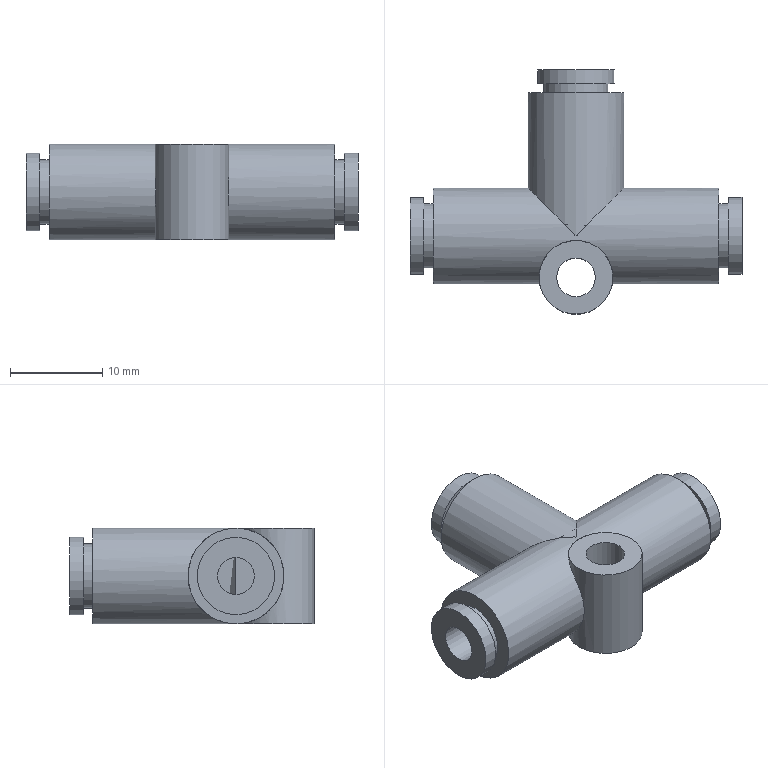Part | NX | 1 solid | 28 faces | box 36 x 26.5 x 10.4 mm | volume 3485 mm3 | plane 14 | cylinder 13 | cone 1 | commonest cylinder face diameters 4 x3 7 x3 8.4 x3 10.4 x2 4.2 x1 8 x1
STEP:
#1=CARTESIAN_POINT('',(0.,0.,5.2));
#2=VERTEX_POINT('',#1);
#3=CARTESIAN_POINT('',(0.,0.,-5.2));
#4=VERTEX_POINT('',#3);
#5=CARTESIAN_POINT('',(0.,0.,0.));
#6=DIRECTION('',(-0.7071,-0.7071,0.));
#7=DIRECTION('',(0.7071,-0.7071,0.));
#8=AXIS2_PLACEMENT_3D('',#5,#6,#7);
#9=ELLIPSE('',#8,7.354,5.2);
#10=EDGE_CURVE('',#2,#4,#9,.T.);
#11=ORIENTED_EDGE('',*,*,#10,.T.);
#12=CARTESIAN_POINT('',(0.,0.,0.));
#13=DIRECTION('',(0.7071,-0.7071,0.));
#14=DIRECTION('',(-0.7071,-0.7071,0.));
#15=AXIS2_PLACEMENT_3D('',#12,#13,#14);
#16=ELLIPSE('',#15,7.354,5.2);
#17=EDGE_CURVE('',#4,#2,#16,.T.);
#18=ORIENTED_EDGE('',*,*,#17,.T.);
#19=EDGE_LOOP('',(#11,#18));
#20=FACE_BOUND('',#19,.T.);
#21=CARTESIAN_POINT('',(-15.5,0.,-5.2));
#22=VERTEX_POINT('',#21);
#23=CARTESIAN_POINT('',(-15.5,0.,0.));
#24=DIRECTION('',(1.,0.,0.));
#25=DIRECTION('',(0.,0.,-1.));
#26=AXIS2_PLACEMENT_3D('',#23,#24,#25);
#27=CIRCLE('',#26,5.2);
#28=EDGE_CURVE('',#22,#22,#27,.T.);
#29=ORIENTED_EDGE('',*,*,#28,.T.);
#30=EDGE_LOOP('',(#29));
#31=FACE_BOUND('',#30,.T.);
#32=CARTESIAN_POINT('',(-4.,-4.5,-2.606));
#33=VERTEX_POINT('',#32);
#34=CARTESIAN_POINT('',(-3.876,-2.858,-4.57));
#35=CARTESIAN_POINT('',(-4.058,-4.689,-2.698));
#36=CARTESIAN_POINT('',(-3.891,-5.385,-0.2717));
#37=CARTESIAN_POINT('',(-4.013,-4.931,2.212));
#38=CARTESIAN_POINT('',(-4.012,-3.327,4.258));
#39=CARTESIAN_POINT('',(-2.719,-1.208,5.153));
#40=CARTESIAN_POINT('',(-0.2808,-0.2446,5.177));
#41=CARTESIAN_POINT('',(2.249,-0.8668,5.188));
#42=CARTESIAN_POINT('',(3.874,-2.854,4.572));
#43=CARTESIAN_POINT('',(4.059,-4.685,2.705));
#44=CARTESIAN_POINT('',(3.891,-5.385,0.2764));
#45=CARTESIAN_POINT('',(4.013,-4.933,-2.209));
#46=CARTESIAN_POINT('',(4.013,-3.329,-4.257));
#47=CARTESIAN_POINT('',(2.72,-1.207,-5.153));
#48=CARTESIAN_POINT('',(0.2792,-0.2442,-5.177));
#49=CARTESIAN_POINT('',(-2.252,-0.8683,-5.188));
#50=CARTESIAN_POINT('',(-3.876,-2.858,-4.57));
#51=CARTESIAN_POINT('',(-4.058,-4.689,-2.698));
#52=CARTESIAN_POINT('',(-3.891,-5.385,-0.2717));
#53=B_SPLINE_CURVE_WITH_KNOTS('',3,(#34,#35,#36,#37,#38,#39,#40,#41,#42,#43,#44,#45,#46,#47,#48,#49,#50,#51,#52),.UNSPECIFIED.,.T.,.F.,(1,1,1,1,1,1,1,1,1,1,1,1,1,1,1,1,1,1,1,1,1,1,1),(-0.01004,-0.007597,-0.00515,-0.002704,-0.0002574,0.002189,0.004636,0.007082,0.009529,0.01198,0.01442,0.01687,0.01931,0.02176,0.02421,0.02665,0.0291,0.03155,0.03399,0.03644,0.03889,0.04133,0.04378),.UNSPECIFIED.);
#54=EDGE_CURVE('',#33,#33,#53,.T.);
#55=ORIENTED_EDGE('',*,*,#54,.T.);
#56=EDGE_LOOP('',(#55));
#57=FACE_BOUND('',#56,.T.);
#58=CARTESIAN_POINT('',(15.5,0.,-5.2));
#59=VERTEX_POINT('',#58);
#60=CARTESIAN_POINT('',(15.5,0.,0.));
#61=DIRECTION('',(1.,0.,0.));
#62=DIRECTION('',(0.,0.,-1.));
#63=AXIS2_PLACEMENT_3D('',#60,#61,#62);
#64=CIRCLE('',#63,5.2);
#65=EDGE_CURVE('',#59,#59,#64,.F.);
#66=ORIENTED_EDGE('',*,*,#65,.T.);
#67=EDGE_LOOP('',(#66));
#68=FACE_BOUND('',#67,.T.);
#69=CARTESIAN_POINT('',(0.,0.,0.));
#70=DIRECTION('',(1.,0.,0.));
#71=DIRECTION('',(0.,0.,-1.));
#72=AXIS2_PLACEMENT_3D('',#69,#70,#71);
#73=CYLINDRICAL_SURFACE('',#72,5.2);
#74=ADVANCED_FACE('',(#20,#31,#57,#68),#73,.T.);
#75=CARTESIAN_POINT('',(15.5,0.,-3.5));
#76=VERTEX_POINT('',#75);
#77=CARTESIAN_POINT('',(15.5,0.,0.));
#78=DIRECTION('',(1.,0.,0.));
#79=DIRECTION('',(0.,0.,-1.));
#80=AXIS2_PLACEMENT_3D('',#77,#78,#79);
#81=CIRCLE('',#80,3.5);
#82=EDGE_CURVE('',#76,#76,#81,.F.);
#83=ORIENTED_EDGE('',*,*,#82,.T.);
#84=EDGE_LOOP('',(#83));
#85=FACE_BOUND('',#84,.T.);
#86=ORIENTED_EDGE('',*,*,#65,.F.);
#87=EDGE_LOOP('',(#86));
#88=FACE_BOUND('',#87,.T.);
#89=CARTESIAN_POINT('',(15.5,4.35,0.));
#90=DIRECTION('',(1.,0.,0.));
#91=DIRECTION('',(0.,0.,-1.));
#92=AXIS2_PLACEMENT_3D('',#89,#90,#91);
#93=PLANE('',#92);
#94=ADVANCED_FACE('',(#85,#88),#93,.T.);
#95=CARTESIAN_POINT('',(4.,-4.5,5.2));
#96=VERTEX_POINT('',#95);
#97=CARTESIAN_POINT('',(0.,-4.5,5.2));
#98=DIRECTION('',(0.,0.,1.));
#99=DIRECTION('',(1.,0.,0.));
#100=AXIS2_PLACEMENT_3D('',#97,#98,#99);
#101=CIRCLE('',#100,4.);
#102=EDGE_CURVE('',#96,#96,#101,.F.);
#103=ORIENTED_EDGE('',*,*,#102,.T.);
#104=EDGE_LOOP('',(#103));
#105=FACE_BOUND('',#104,.T.);
#106=CARTESIAN_POINT('',(4.,-4.5,-5.2));
#107=VERTEX_POINT('',#106);
#108=CARTESIAN_POINT('',(0.,-4.5,-5.2));
#109=DIRECTION('',(0.,0.,1.));
#110=DIRECTION('',(1.,0.,0.));
#111=AXIS2_PLACEMENT_3D('',#108,#109,#110);
#112=CIRCLE('',#111,4.);
#113=EDGE_CURVE('',#107,#107,#112,.T.);
#114=ORIENTED_EDGE('',*,*,#113,.T.);
#115=EDGE_LOOP('',(#114));
#116=FACE_BOUND('',#115,.T.);
#117=ORIENTED_EDGE('',*,*,#54,.F.);
#118=EDGE_LOOP('',(#117));
#119=FACE_BOUND('',#118,.T.);
#120=CARTESIAN_POINT('',(0.,-4.5,5.2));
#121=DIRECTION('',(0.,0.,1.));
#122=DIRECTION('',(1.,0.,0.));
#123=AXIS2_PLACEMENT_3D('',#120,#121,#122);
#124=CYLINDRICAL_SURFACE('',#123,4.);
#125=ADVANCED_FACE('',(#105,#116,#119),#124,.T.);
#126=ORIENTED_EDGE('',*,*,#28,.F.);
#127=EDGE_LOOP('',(#126));
#128=FACE_BOUND('',#127,.T.);
#129=CARTESIAN_POINT('',(-15.5,0.,-3.5));
#130=VERTEX_POINT('',#129);
#131=CARTESIAN_POINT('',(-15.5,0.,0.));
#132=DIRECTION('',(1.,0.,0.));
#133=DIRECTION('',(0.,0.,-1.));
#134=AXIS2_PLACEMENT_3D('',#131,#132,#133);
#135=CIRCLE('',#134,3.5);
#136=EDGE_CURVE('',#130,#130,#135,.T.);
#137=ORIENTED_EDGE('',*,*,#136,.T.);
#138=EDGE_LOOP('',(#137));
#139=FACE_BOUND('',#138,.T.);
#140=CARTESIAN_POINT('',(-15.5,4.35,0.));
#141=DIRECTION('',(-1.,0.,0.));
#142=DIRECTION('',(0.,0.,1.));
#143=AXIS2_PLACEMENT_3D('',#140,#141,#142);
#144=PLANE('',#143);
#145=ADVANCED_FACE('',(#128,#139),#144,.T.);
#146=CARTESIAN_POINT('',(0.,15.5,-5.2));
#147=VERTEX_POINT('',#146);
#148=CARTESIAN_POINT('',(0.,15.5,0.));
#149=DIRECTION('',(0.,-1.,0.));
#150=DIRECTION('',(0.,0.,-1.));
#151=AXIS2_PLACEMENT_3D('',#148,#149,#150);
#152=CIRCLE('',#151,5.2);
#153=EDGE_CURVE('',#147,#147,#152,.T.);
#154=ORIENTED_EDGE('',*,*,#153,.T.);
#155=EDGE_LOOP('',(#154));
#156=FACE_BOUND('',#155,.T.);
#157=ORIENTED_EDGE('',*,*,#10,.F.);
#158=ORIENTED_EDGE('',*,*,#17,.F.);
#159=EDGE_LOOP('',(#157,#158));
#160=FACE_BOUND('',#159,.T.);
#161=CARTESIAN_POINT('',(0.,7.75,0.));
#162=DIRECTION('',(0.,-1.,0.));
#163=DIRECTION('',(0.,0.,-1.));
#164=AXIS2_PLACEMENT_3D('',#161,#162,#163);
#165=CYLINDRICAL_SURFACE('',#164,5.2);
#166=ADVANCED_FACE('',(#156,#160),#165,.T.);
#167=ORIENTED_EDGE('',*,*,#82,.F.);
#168=EDGE_LOOP('',(#167));
#169=FACE_BOUND('',#168,.T.);
#170=CARTESIAN_POINT('',(16.5,0.,-3.5));
#171=VERTEX_POINT('',#170);
#172=CARTESIAN_POINT('',(16.5,0.,0.));
#173=DIRECTION('',(1.,0.,0.));
#174=DIRECTION('',(0.,0.,-1.));
#175=AXIS2_PLACEMENT_3D('',#172,#173,#174);
#176=CIRCLE('',#175,3.5);
#177=EDGE_CURVE('',#171,#171,#176,.F.);
#178=ORIENTED_EDGE('',*,*,#177,.T.);
#179=EDGE_LOOP('',(#178));
#180=FACE_BOUND('',#179,.T.);
#181=CARTESIAN_POINT('',(16.,0.,0.));
#182=DIRECTION('',(1.,0.,0.));
#183=DIRECTION('',(0.,0.,-1.));
#184=AXIS2_PLACEMENT_3D('',#181,#182,#183);
#185=CYLINDRICAL_SURFACE('',#184,3.5);
#186=ADVANCED_FACE('',(#169,#180),#185,.T.);
#187=ORIENTED_EDGE('',*,*,#113,.F.);
#188=EDGE_LOOP('',(#187));
#189=FACE_BOUND('',#188,.T.);
#190=CARTESIAN_POINT('',(2.1,-4.5,-5.2));
#191=VERTEX_POINT('',#190);
#192=CARTESIAN_POINT('',(0.,-4.5,-5.2));
#193=DIRECTION('',(0.,0.,1.));
#194=DIRECTION('',(1.,0.,0.));
#195=AXIS2_PLACEMENT_3D('',#192,#193,#194);
#196=CIRCLE('',#195,2.1);
#197=EDGE_CURVE('',#191,#191,#196,.F.);
#198=ORIENTED_EDGE('',*,*,#197,.F.);
#199=EDGE_LOOP('',(#198));
#200=FACE_BOUND('',#199,.T.);
#201=CARTESIAN_POINT('',(0.,0.,-5.2));
#202=DIRECTION('',(0.,0.,1.));
#203=DIRECTION('',(1.,0.,0.));
#204=AXIS2_PLACEMENT_3D('',#201,#202,#203);
#205=PLANE('',#204);
#206=ADVANCED_FACE('',(#189,#200),#205,.F.);
#207=ORIENTED_EDGE('',*,*,#102,.F.);
#208=EDGE_LOOP('',(#207));
#209=FACE_BOUND('',#208,.T.);
#210=CARTESIAN_POINT('',(2.1,-4.5,5.2));
#211=VERTEX_POINT('',#210);
#212=CARTESIAN_POINT('',(0.,-4.5,5.2));
#213=DIRECTION('',(0.,0.,1.));
#214=DIRECTION('',(1.,0.,0.));
#215=AXIS2_PLACEMENT_3D('',#212,#213,#214);
#216=CIRCLE('',#215,2.1);
#217=EDGE_CURVE('',#211,#211,#216,.F.);
#218=ORIENTED_EDGE('',*,*,#217,.T.);
#219=EDGE_LOOP('',(#218));
#220=FACE_BOUND('',#219,.T.);
#221=CARTESIAN_POINT('',(0.,0.,5.2));
#222=DIRECTION('',(0.,0.,1.));
#223=DIRECTION('',(1.,0.,0.));
#224=AXIS2_PLACEMENT_3D('',#221,#222,#223);
#225=PLANE('',#224);
#226=ADVANCED_FACE('',(#209,#220),#225,.T.);
#227=CARTESIAN_POINT('',(-16.5,0.,-3.5));
#228=VERTEX_POINT('',#227);
#229=CARTESIAN_POINT('',(-16.5,0.,0.));
#230=DIRECTION('',(1.,0.,0.));
#231=DIRECTION('',(0.,0.,-1.));
#232=AXIS2_PLACEMENT_3D('',#229,#230,#231);
#233=CIRCLE('',#232,3.5);
#234=EDGE_CURVE('',#228,#228,#233,.T.);
#235=ORIENTED_EDGE('',*,*,#234,.T.);
#236=EDGE_LOOP('',(#235));
#237=FACE_BOUND('',#236,.T.);
#238=ORIENTED_EDGE('',*,*,#136,.F.);
#239=EDGE_LOOP('',(#238));
#240=FACE_BOUND('',#239,.T.);
#241=CARTESIAN_POINT('',(-16.,0.,0.));
#242=DIRECTION('',(1.,0.,0.));
#243=DIRECTION('',(0.,0.,-1.));
#244=AXIS2_PLACEMENT_3D('',#241,#242,#243);
#245=CYLINDRICAL_SURFACE('',#244,3.5);
#246=ADVANCED_FACE('',(#237,#240),#245,.T.);
#247=ORIENTED_EDGE('',*,*,#153,.F.);
#248=EDGE_LOOP('',(#247));
#249=FACE_BOUND('',#248,.T.);
#250=CARTESIAN_POINT('',(0.,15.5,-3.5));
#251=VERTEX_POINT('',#250);
#252=CARTESIAN_POINT('',(0.,15.5,0.));
#253=DIRECTION('',(0.,-1.,0.));
#254=DIRECTION('',(0.,0.,-1.));
#255=AXIS2_PLACEMENT_3D('',#252,#253,#254);
#256=CIRCLE('',#255,3.5);
#257=EDGE_CURVE('',#251,#251,#256,.T.);
#258=ORIENTED_EDGE('',*,*,#257,.T.);
#259=EDGE_LOOP('',(#258));
#260=FACE_BOUND('',#259,.T.);
#261=CARTESIAN_POINT('',(4.35,15.5,0.));
#262=DIRECTION('',(0.,1.,0.));
#263=DIRECTION('',(0.,0.,1.));
#264=AXIS2_PLACEMENT_3D('',#261,#262,#263);
#265=PLANE('',#264);
#266=ADVANCED_FACE('',(#249,#260),#265,.T.);
#267=CARTESIAN_POINT('',(16.5,0.,-4.2));
#268=VERTEX_POINT('',#267);
#269=CARTESIAN_POINT('',(16.5,0.,0.));
#270=DIRECTION('',(1.,0.,0.));
#271=DIRECTION('',(0.,0.,-1.));
#272=AXIS2_PLACEMENT_3D('',#269,#270,#271);
#273=CIRCLE('',#272,4.2);
#274=EDGE_CURVE('',#268,#268,#273,.F.);
#275=ORIENTED_EDGE('',*,*,#274,.T.);
#276=EDGE_LOOP('',(#275));
#277=FACE_BOUND('',#276,.T.);
#278=ORIENTED_EDGE('',*,*,#177,.F.);
#279=EDGE_LOOP('',(#278));
#280=FACE_BOUND('',#279,.T.);
#281=CARTESIAN_POINT('',(16.5,3.85,0.));
#282=DIRECTION('',(-1.,0.,0.));
#283=DIRECTION('',(0.,0.,1.));
#284=AXIS2_PLACEMENT_3D('',#281,#282,#283);
#285=PLANE('',#284);
#286=ADVANCED_FACE('',(#277,#280),#285,.T.);
#287=ORIENTED_EDGE('',*,*,#197,.T.);
#288=EDGE_LOOP('',(#287));
#289=FACE_BOUND('',#288,.T.);
#290=ORIENTED_EDGE('',*,*,#217,.F.);
#291=EDGE_LOOP('',(#290));
#292=FACE_BOUND('',#291,.T.);
#293=CARTESIAN_POINT('',(0.,-4.5,5.2));
#294=DIRECTION('',(0.,0.,1.));
#295=DIRECTION('',(1.,0.,0.));
#296=AXIS2_PLACEMENT_3D('',#293,#294,#295);
#297=CYLINDRICAL_SURFACE('',#296,2.1);
#298=ADVANCED_FACE('',(#289,#292),#297,.F.);
#299=ORIENTED_EDGE('',*,*,#234,.F.);
#300=EDGE_LOOP('',(#299));
#301=FACE_BOUND('',#300,.T.);
#302=CARTESIAN_POINT('',(-16.5,0.,-4.2));
#303=VERTEX_POINT('',#302);
#304=CARTESIAN_POINT('',(-16.5,0.,0.));
#305=DIRECTION('',(1.,0.,0.));
#306=DIRECTION('',(0.,0.,-1.));
#307=AXIS2_PLACEMENT_3D('',#304,#305,#306);
#308=CIRCLE('',#307,4.2);
#309=EDGE_CURVE('',#303,#303,#308,.T.);
#310=ORIENTED_EDGE('',*,*,#309,.T.);
#311=EDGE_LOOP('',(#310));
#312=FACE_BOUND('',#311,.T.);
#313=CARTESIAN_POINT('',(-16.5,3.85,0.));
#314=DIRECTION('',(1.,0.,0.));
#315=DIRECTION('',(0.,0.,-1.));
#316=AXIS2_PLACEMENT_3D('',#313,#314,#315);
#317=PLANE('',#316);
#318=ADVANCED_FACE('',(#301,#312),#317,.T.);
#319=CARTESIAN_POINT('',(0.,16.5,-3.5));
#320=VERTEX_POINT('',#319);
#321=CARTESIAN_POINT('',(0.,16.5,0.));
#322=DIRECTION('',(0.,-1.,0.));
#323=DIRECTION('',(0.,0.,-1.));
#324=AXIS2_PLACEMENT_3D('',#321,#322,#323);
#325=CIRCLE('',#324,3.5);
#326=EDGE_CURVE('',#320,#320,#325,.T.);
#327=ORIENTED_EDGE('',*,*,#326,.T.);
#328=EDGE_LOOP('',(#327));
#329=FACE_BOUND('',#328,.T.);
#330=ORIENTED_EDGE('',*,*,#257,.F.);
#331=EDGE_LOOP('',(#330));
#332=FACE_BOUND('',#331,.T.);
#333=CARTESIAN_POINT('',(0.,16.,0.));
#334=DIRECTION('',(0.,-1.,0.));
#335=DIRECTION('',(0.,0.,-1.));
#336=AXIS2_PLACEMENT_3D('',#333,#334,#335);
#337=CYLINDRICAL_SURFACE('',#336,3.5);
#338=ADVANCED_FACE('',(#329,#332),#337,.T.);
#339=ORIENTED_EDGE('',*,*,#274,.F.);
#340=EDGE_LOOP('',(#339));
#341=FACE_BOUND('',#340,.T.);
#342=CARTESIAN_POINT('',(18.,0.,-4.2));
#343=VERTEX_POINT('',#342);
#344=CARTESIAN_POINT('',(18.,0.,0.));
#345=DIRECTION('',(1.,0.,0.));
#346=DIRECTION('',(0.,0.,-1.));
#347=AXIS2_PLACEMENT_3D('',#344,#345,#346);
#348=CIRCLE('',#347,4.2);
#349=EDGE_CURVE('',#343,#343,#348,.F.);
#350=ORIENTED_EDGE('',*,*,#349,.T.);
#351=EDGE_LOOP('',(#350));
#352=FACE_BOUND('',#351,.T.);
#353=CARTESIAN_POINT('',(17.25,0.,0.));
#354=DIRECTION('',(1.,0.,0.));
#355=DIRECTION('',(0.,0.,-1.));
#356=AXIS2_PLACEMENT_3D('',#353,#354,#355);
#357=CYLINDRICAL_SURFACE('',#356,4.2);
#358=ADVANCED_FACE('',(#341,#352),#357,.T.);
#359=CARTESIAN_POINT('',(-18.,0.,-4.2));
#360=VERTEX_POINT('',#359);
#361=CARTESIAN_POINT('',(-18.,0.,0.));
#362=DIRECTION('',(1.,0.,0.));
#363=DIRECTION('',(0.,0.,-1.));
#364=AXIS2_PLACEMENT_3D('',#361,#362,#363);
#365=CIRCLE('',#364,4.2);
#366=EDGE_CURVE('',#360,#360,#365,.T.);
#367=ORIENTED_EDGE('',*,*,#366,.T.);
#368=EDGE_LOOP('',(#367));
#369=FACE_BOUND('',#368,.T.);
#370=ORIENTED_EDGE('',*,*,#309,.F.);
#371=EDGE_LOOP('',(#370));
#372=FACE_BOUND('',#371,.T.);
#373=CARTESIAN_POINT('',(-17.25,0.,0.));
#374=DIRECTION('',(1.,0.,0.));
#375=DIRECTION('',(0.,0.,-1.));
#376=AXIS2_PLACEMENT_3D('',#373,#374,#375);
#377=CYLINDRICAL_SURFACE('',#376,4.2);
#378=ADVANCED_FACE('',(#369,#372),#377,.T.);
#379=ORIENTED_EDGE('',*,*,#326,.F.);
#380=EDGE_LOOP('',(#379));
#381=FACE_BOUND('',#380,.T.);
#382=CARTESIAN_POINT('',(0.,16.5,-4.2));
#383=VERTEX_POINT('',#382);
#384=CARTESIAN_POINT('',(0.,16.5,0.));
#385=DIRECTION('',(0.,-1.,0.));
#386=DIRECTION('',(0.,0.,-1.));
#387=AXIS2_PLACEMENT_3D('',#384,#385,#386);
#388=CIRCLE('',#387,4.2);
#389=EDGE_CURVE('',#383,#383,#388,.T.);
#390=ORIENTED_EDGE('',*,*,#389,.T.);
#391=EDGE_LOOP('',(#390));
#392=FACE_BOUND('',#391,.T.);
#393=CARTESIAN_POINT('',(3.85,16.5,0.));
#394=DIRECTION('',(0.,-1.,0.));
#395=DIRECTION('',(0.,0.,-1.));
#396=AXIS2_PLACEMENT_3D('',#393,#394,#395);
#397=PLANE('',#396);
#398=ADVANCED_FACE('',(#381,#392),#397,.T.);
#399=ORIENTED_EDGE('',*,*,#349,.F.);
#400=EDGE_LOOP('',(#399));
#401=FACE_BOUND('',#400,.T.);
#402=CARTESIAN_POINT('',(18.,0.,-2.));
#403=VERTEX_POINT('',#402);
#404=CARTESIAN_POINT('',(18.,0.,0.));
#405=DIRECTION('',(1.,0.,0.));
#406=DIRECTION('',(0.,0.,-1.));
#407=AXIS2_PLACEMENT_3D('',#404,#405,#406);
#408=CIRCLE('',#407,2.);
#409=EDGE_CURVE('',#403,#403,#408,.F.);
#410=ORIENTED_EDGE('',*,*,#409,.T.);
#411=EDGE_LOOP('',(#410));
#412=FACE_BOUND('',#411,.T.);
#413=CARTESIAN_POINT('',(18.,2.1,0.));
#414=DIRECTION('',(1.,0.,0.));
#415=DIRECTION('',(0.,0.,-1.));
#416=AXIS2_PLACEMENT_3D('',#413,#414,#415);
#417=PLANE('',#416);
#418=ADVANCED_FACE('',(#401,#412),#417,.T.);
#419=ORIENTED_EDGE('',*,*,#366,.F.);
#420=EDGE_LOOP('',(#419));
#421=FACE_BOUND('',#420,.T.);
#422=CARTESIAN_POINT('',(-18.,0.,2.));
#423=VERTEX_POINT('',#422);
#424=CARTESIAN_POINT('',(-18.,0.,0.));
#425=DIRECTION('',(-1.,0.,0.));
#426=DIRECTION('',(0.,0.,1.));
#427=AXIS2_PLACEMENT_3D('',#424,#425,#426);
#428=CIRCLE('',#427,2.);
#429=EDGE_CURVE('',#423,#423,#428,.F.);
#430=ORIENTED_EDGE('',*,*,#429,.T.);
#431=EDGE_LOOP('',(#430));
#432=FACE_BOUND('',#431,.T.);
#433=CARTESIAN_POINT('',(-18.,2.1,0.));
#434=DIRECTION('',(-1.,0.,0.));
#435=DIRECTION('',(0.,0.,1.));
#436=AXIS2_PLACEMENT_3D('',#433,#434,#435);
#437=PLANE('',#436);
#438=ADVANCED_FACE('',(#421,#432),#437,.T.);
#439=CARTESIAN_POINT('',(0.,18.,-4.2));
#440=VERTEX_POINT('',#439);
#441=CARTESIAN_POINT('',(0.,18.,0.));
#442=DIRECTION('',(0.,-1.,0.));
#443=DIRECTION('',(0.,0.,-1.));
#444=AXIS2_PLACEMENT_3D('',#441,#442,#443);
#445=CIRCLE('',#444,4.2);
#446=EDGE_CURVE('',#440,#440,#445,.T.);
#447=ORIENTED_EDGE('',*,*,#446,.T.);
#448=EDGE_LOOP('',(#447));
#449=FACE_BOUND('',#448,.T.);
#450=ORIENTED_EDGE('',*,*,#389,.F.);
#451=EDGE_LOOP('',(#450));
#452=FACE_BOUND('',#451,.T.);
#453=CARTESIAN_POINT('',(0.,17.25,0.));
#454=DIRECTION('',(0.,-1.,0.));
#455=DIRECTION('',(0.,0.,-1.));
#456=AXIS2_PLACEMENT_3D('',#453,#454,#455);
#457=CYLINDRICAL_SURFACE('',#456,4.2);
#458=ADVANCED_FACE('',(#449,#452),#457,.T.);
#459=ORIENTED_EDGE('',*,*,#409,.F.);
#460=EDGE_LOOP('',(#459));
#461=FACE_BOUND('',#460,.T.);
#462=CARTESIAN_POINT('',(2.,0.,-2.));
#463=VERTEX_POINT('',#462);
#464=CARTESIAN_POINT('',(2.,0.,0.));
#465=DIRECTION('',(1.,0.,0.));
#466=DIRECTION('',(0.,0.,-1.));
#467=AXIS2_PLACEMENT_3D('',#464,#465,#466);
#468=CIRCLE('',#467,2.);
#469=EDGE_CURVE('',#463,#463,#468,.T.);
#470=ORIENTED_EDGE('',*,*,#469,.F.);
#471=EDGE_LOOP('',(#470));
#472=FACE_BOUND('',#471,.T.);
#473=CARTESIAN_POINT('',(18.,0.,0.));
#474=DIRECTION('',(1.,0.,0.));
#475=DIRECTION('',(0.,0.,-1.));
#476=AXIS2_PLACEMENT_3D('',#473,#474,#475);
#477=CYLINDRICAL_SURFACE('',#476,2.);
#478=ADVANCED_FACE('',(#461,#472),#477,.F.);
#479=ORIENTED_EDGE('',*,*,#429,.F.);
#480=EDGE_LOOP('',(#479));
#481=FACE_BOUND('',#480,.T.);
#482=CARTESIAN_POINT('',(-2.,0.,2.));
#483=VERTEX_POINT('',#482);
#484=CARTESIAN_POINT('',(-2.,0.,0.));
#485=DIRECTION('',(-1.,0.,0.));
#486=DIRECTION('',(0.,0.,1.));
#487=AXIS2_PLACEMENT_3D('',#484,#485,#486);
#488=CIRCLE('',#487,2.);
#489=EDGE_CURVE('',#483,#483,#488,.T.);
#490=ORIENTED_EDGE('',*,*,#489,.F.);
#491=EDGE_LOOP('',(#490));
#492=FACE_BOUND('',#491,.T.);
#493=CARTESIAN_POINT('',(-18.,0.,0.));
#494=DIRECTION('',(-1.,0.,0.));
#495=DIRECTION('',(0.,0.,1.));
#496=AXIS2_PLACEMENT_3D('',#493,#494,#495);
#497=CYLINDRICAL_SURFACE('',#496,2.);
#498=ADVANCED_FACE('',(#481,#492),#497,.F.);
#499=ORIENTED_EDGE('',*,*,#446,.F.);
#500=EDGE_LOOP('',(#499));
#501=FACE_BOUND('',#500,.T.);
#502=CARTESIAN_POINT('',(0.,18.,-2.));
#503=VERTEX_POINT('',#502);
#504=CARTESIAN_POINT('',(0.,18.,0.));
#505=DIRECTION('',(0.,-1.,0.));
#506=DIRECTION('',(0.,0.,-1.));
#507=AXIS2_PLACEMENT_3D('',#504,#505,#506);
#508=CIRCLE('',#507,2.);
#509=EDGE_CURVE('',#503,#503,#508,.T.);
#510=ORIENTED_EDGE('',*,*,#509,.T.);
#511=EDGE_LOOP('',(#510));
#512=FACE_BOUND('',#511,.T.);
#513=CARTESIAN_POINT('',(2.1,18.,0.));
#514=DIRECTION('',(0.,1.,0.));
#515=DIRECTION('',(0.,0.,1.));
#516=AXIS2_PLACEMENT_3D('',#513,#514,#515);
#517=PLANE('',#516);
#518=ADVANCED_FACE('',(#501,#512),#517,.T.);
#519=ORIENTED_EDGE('',*,*,#469,.T.);
#520=EDGE_LOOP('',(#519));
#521=FACE_BOUND('',#520,.T.);
#522=CARTESIAN_POINT('',(2.,0.,0.));
#523=DIRECTION('',(1.,0.,0.));
#524=DIRECTION('',(0.,0.,-1.));
#525=AXIS2_PLACEMENT_3D('',#522,#523,#524);
#526=PLANE('',#525);
#527=ADVANCED_FACE('',(#521),#526,.T.);
#528=ORIENTED_EDGE('',*,*,#489,.T.);
#529=EDGE_LOOP('',(#528));
#530=FACE_BOUND('',#529,.T.);
#531=CARTESIAN_POINT('',(-2.,0.,0.));
#532=DIRECTION('',(-1.,0.,0.));
#533=DIRECTION('',(0.,0.,1.));
#534=AXIS2_PLACEMENT_3D('',#531,#532,#533);
#535=PLANE('',#534);
#536=ADVANCED_FACE('',(#530),#535,.T.);
#537=ORIENTED_EDGE('',*,*,#509,.F.);
#538=EDGE_LOOP('',(#537));
#539=FACE_BOUND('',#538,.T.);
#540=CARTESIAN_POINT('',(0.,2.1,-2.));
#541=VERTEX_POINT('',#540);
#542=CARTESIAN_POINT('',(0.,2.1,0.));
#543=DIRECTION('',(0.,-1.,0.));
#544=DIRECTION('',(0.,0.,-1.));
#545=AXIS2_PLACEMENT_3D('',#542,#543,#544);
#546=CIRCLE('',#545,2.);
#547=EDGE_CURVE('',#541,#541,#546,.F.);
#548=ORIENTED_EDGE('',*,*,#547,.F.);
#549=EDGE_LOOP('',(#548));
#550=FACE_BOUND('',#549,.T.);
#551=CARTESIAN_POINT('',(0.,10.05,0.));
#552=DIRECTION('',(0.,-1.,0.));
#553=DIRECTION('',(0.,0.,-1.));
#554=AXIS2_PLACEMENT_3D('',#551,#552,#553);
#555=CYLINDRICAL_SURFACE('',#554,2.);
#556=ADVANCED_FACE('',(#539,#550),#555,.F.);
#557=ORIENTED_EDGE('',*,*,#547,.T.);
#558=EDGE_LOOP('',(#557));
#559=FACE_BOUND('',#558,.T.);
#560=CARTESIAN_POINT('',(0.,2.,1.9));
#561=VERTEX_POINT('',#560);
#562=CARTESIAN_POINT('',(0.,2.,0.));
#563=DIRECTION('',(0.,1.,0.));
#564=DIRECTION('',(0.,0.,1.));
#565=AXIS2_PLACEMENT_3D('',#562,#563,#564);
#566=CIRCLE('',#565,1.9);
#567=EDGE_CURVE('',#561,#561,#566,.T.);
#568=ORIENTED_EDGE('',*,*,#567,.F.);
#569=EDGE_LOOP('',(#568));
#570=FACE_BOUND('',#569,.T.);
#571=CARTESIAN_POINT('',(0.,2.1,0.));
#572=DIRECTION('',(0.,1.,0.));
#573=DIRECTION('',(0.,0.,1.));
#574=AXIS2_PLACEMENT_3D('',#571,#572,#573);
#575=CONICAL_SURFACE('',#574,2.,0.7854);
#576=ADVANCED_FACE('',(#559,#570),#575,.F.);
#577=ORIENTED_EDGE('',*,*,#567,.T.);
#578=EDGE_LOOP('',(#577));
#579=FACE_BOUND('',#578,.T.);
#580=CARTESIAN_POINT('',(0.95,2.,0.));
#581=DIRECTION('',(0.,-1.,0.));
#582=DIRECTION('',(0.,0.,-1.));
#583=AXIS2_PLACEMENT_3D('',#580,#581,#582);
#584=PLANE('',#583);
#585=ADVANCED_FACE('',(#579),#584,.F.);
#586=CLOSED_SHELL('',(#74,#94,#125,#145,#166,#186,#206,#226,#246,#266,#286,#298,#318,#338,#358,#378,#398,#418,#438,#458,#478,#498,#518,#527,#536,#556,#576,#585));
#587=MANIFOLD_SOLID_BREP('',#586);
#588=(LENGTH_UNIT()NAMED_UNIT(*)SI_UNIT(.MILLI.,.METRE.));
#589=UNCERTAINTY_MEASURE_WITH_UNIT(LENGTH_MEASURE(0.0508),#588,'','');
#590=(NAMED_UNIT(*)PLANE_ANGLE_UNIT()SI_UNIT($,.RADIAN.));
#591=(NAMED_UNIT(*)SI_UNIT($,.STERADIAN.)SOLID_ANGLE_UNIT());
#592=(GEOMETRIC_REPRESENTATION_CONTEXT(3)GLOBAL_UNCERTAINTY_ASSIGNED_CONTEXT((#589))GLOBAL_UNIT_ASSIGNED_CONTEXT((#588,#590,#591))REPRESENTATION_CONTEXT('',''));
#593=ADVANCED_BREP_SHAPE_REPRESENTATION('',(#587),#592);